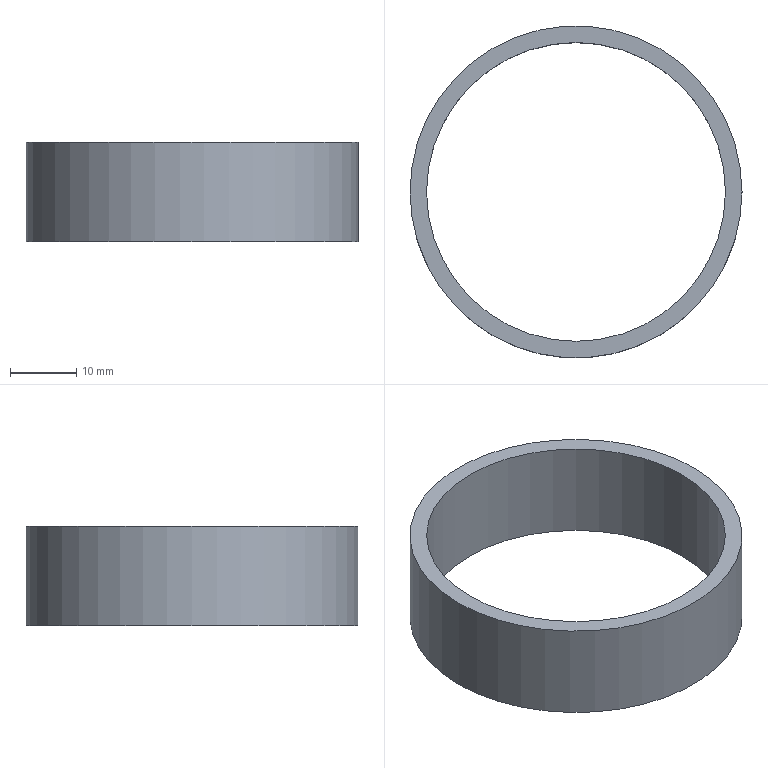Part | NX | features DATUM_CSYS 2, EXTRUDE 1, SKETCH 1 | 1 solid | 4 faces | box 50 x 50 x 15 mm | volume 5596 mm3 | cylinder 2 | plane 2 | commonest cylinder face diameters 45 x1 50 x1
STEP:
#1=CARTESIAN_POINT('',(25.,0.,15.));
#2=VERTEX_POINT('',#1);
#3=CARTESIAN_POINT('',(0.,0.,15.));
#4=DIRECTION('',(0.,0.,1.));
#5=DIRECTION('',(1.,0.,0.));
#6=AXIS2_PLACEMENT_3D('',#3,#4,#5);
#7=CIRCLE('',#6,25.);
#8=EDGE_CURVE('',#2,#2,#7,.T.);
#9=ORIENTED_EDGE('',*,*,#8,.F.);
#10=EDGE_LOOP('',(#9));
#11=FACE_BOUND('',#10,.T.);
#12=CARTESIAN_POINT('',(25.,0.,0.));
#13=VERTEX_POINT('',#12);
#14=CARTESIAN_POINT('',(0.,0.,0.));
#15=DIRECTION('',(0.,0.,1.));
#16=DIRECTION('',(1.,0.,0.));
#17=AXIS2_PLACEMENT_3D('',#14,#15,#16);
#18=CIRCLE('',#17,25.);
#19=EDGE_CURVE('',#13,#13,#18,.T.);
#20=ORIENTED_EDGE('',*,*,#19,.T.);
#21=EDGE_LOOP('',(#20));
#22=FACE_BOUND('',#21,.T.);
#23=CARTESIAN_POINT('',(0.,0.,15.));
#24=DIRECTION('',(0.,0.,-1.));
#25=DIRECTION('',(-1.,0.,0.));
#26=AXIS2_PLACEMENT_3D('',#23,#24,#25);
#27=CYLINDRICAL_SURFACE('',#26,25.);
#28=ADVANCED_FACE('',(#11,#22),#27,.T.);
#29=CARTESIAN_POINT('',(22.5,0.,15.));
#30=VERTEX_POINT('',#29);
#31=CARTESIAN_POINT('',(0.,0.,15.));
#32=DIRECTION('',(0.,0.,1.));
#33=DIRECTION('',(1.,0.,0.));
#34=AXIS2_PLACEMENT_3D('',#31,#32,#33);
#35=CIRCLE('',#34,22.5);
#36=EDGE_CURVE('',#30,#30,#35,.T.);
#37=ORIENTED_EDGE('',*,*,#36,.T.);
#38=EDGE_LOOP('',(#37));
#39=FACE_BOUND('',#38,.T.);
#40=CARTESIAN_POINT('',(22.5,0.,0.));
#41=VERTEX_POINT('',#40);
#42=CARTESIAN_POINT('',(0.,0.,0.));
#43=DIRECTION('',(0.,0.,1.));
#44=DIRECTION('',(1.,0.,0.));
#45=AXIS2_PLACEMENT_3D('',#42,#43,#44);
#46=CIRCLE('',#45,22.5);
#47=EDGE_CURVE('',#41,#41,#46,.T.);
#48=ORIENTED_EDGE('',*,*,#47,.F.);
#49=EDGE_LOOP('',(#48));
#50=FACE_BOUND('',#49,.T.);
#51=CARTESIAN_POINT('',(0.,0.,15.));
#52=DIRECTION('',(0.,0.,-1.));
#53=DIRECTION('',(-1.,0.,0.));
#54=AXIS2_PLACEMENT_3D('',#51,#52,#53);
#55=CYLINDRICAL_SURFACE('',#54,22.5);
#56=ADVANCED_FACE('',(#39,#50),#55,.F.);
#57=ORIENTED_EDGE('',*,*,#8,.T.);
#58=EDGE_LOOP('',(#57));
#59=FACE_BOUND('',#58,.T.);
#60=ORIENTED_EDGE('',*,*,#36,.F.);
#61=EDGE_LOOP('',(#60));
#62=FACE_BOUND('',#61,.T.);
#63=CARTESIAN_POINT('',(0.,0.,15.));
#64=DIRECTION('',(0.,0.,1.));
#65=DIRECTION('',(1.,0.,0.));
#66=AXIS2_PLACEMENT_3D('',#63,#64,#65);
#67=PLANE('',#66);
#68=ADVANCED_FACE('',(#59,#62),#67,.T.);
#69=ORIENTED_EDGE('',*,*,#19,.F.);
#70=EDGE_LOOP('',(#69));
#71=FACE_BOUND('',#70,.T.);
#72=ORIENTED_EDGE('',*,*,#47,.T.);
#73=EDGE_LOOP('',(#72));
#74=FACE_BOUND('',#73,.T.);
#75=CARTESIAN_POINT('',(0.,0.,0.));
#76=DIRECTION('',(0.,0.,1.));
#77=DIRECTION('',(1.,0.,0.));
#78=AXIS2_PLACEMENT_3D('',#75,#76,#77);
#79=PLANE('',#78);
#80=ADVANCED_FACE('',(#71,#74),#79,.F.);
#81=CLOSED_SHELL('',(#28,#56,#68,#80));
#82=MANIFOLD_SOLID_BREP('',#81);
#83=(LENGTH_UNIT()NAMED_UNIT(*)SI_UNIT(.MILLI.,.METRE.));
#84=UNCERTAINTY_MEASURE_WITH_UNIT(LENGTH_MEASURE(0.00001),#83,'','');
#85=(NAMED_UNIT(*)PLANE_ANGLE_UNIT()SI_UNIT($,.RADIAN.));
#86=(NAMED_UNIT(*)SI_UNIT($,.STERADIAN.)SOLID_ANGLE_UNIT());
#87=(GEOMETRIC_REPRESENTATION_CONTEXT(3)GLOBAL_UNCERTAINTY_ASSIGNED_CONTEXT((#84))GLOBAL_UNIT_ASSIGNED_CONTEXT((#83,#85,#86))REPRESENTATION_CONTEXT('',''));
#88=ADVANCED_BREP_SHAPE_REPRESENTATION('',(#82),#87);